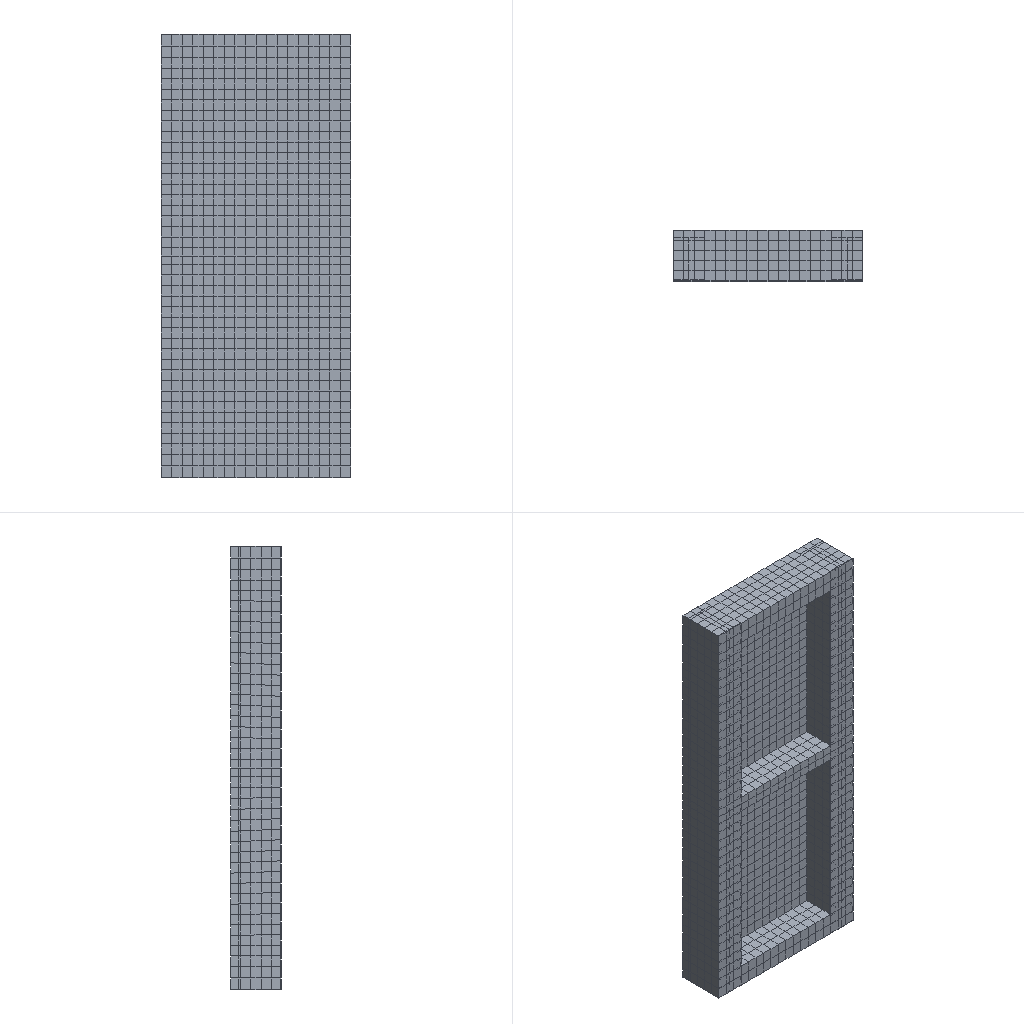Simulation study | abaqus
Set-up summary:
category,name,step,type,value,unit,region
solver,abaqus
solver,version,,,Abaqus/Explicit 2020
units,not stated in the deck,,not stated
analysis,deck,,transient,transient
load_step,Step-1,Step-1,transient
load_step,requested,,,1
mesh,nodes,,,5312
mesh,elements,,,3890
element_type,S4R,,shell,1008
element_type,T3D2,,truss,398
element_type,C3D8R,,solid,2484
load,load commands in deck,,count,1
bc,support commands in deck,,count,7
material,CON,,in results
material,STEEL,,in results
check,setup vs results,,match,"per instance, exact: element labels, types and connectivity; labels of the nodes the elements use; coordinates of those nodes at SINGLE_PRECISION in 19 of 19 instance(s)"
Abaqus input file, long lists of numbers shortened:
*Heading
** Job name: Job-3 Model name: Model-2-wangfu
** Generated by: Abaqus/CAE 2020
*Preprint, echo=NO, model=NO, history=NO, contact=NO
**
** PARTS
**
*Part, name=con
*Node
      1,         150.,           0.,        1090.
      2,         150.,           0.,        1350.
** (3778 more lines like these left out)
*Element, type=C3D8R
  1,    1,   73,  793,  106,  162,  849, 2683,  827
  2,   73,   74,  794,  793,  849,  850, 2684, 2683
** (2482 more lines like these left out)
*Nset, nset=Set-1, generate
    1,  3780,     1
*Elset, elset=Set-1, generate
    1,  2484,     1
** Section: con
*Solid Section, elset=Set-1, material=con
,
*End Part
**
*Part, name=gong
*Node
      1,           0.,           0.,           0.
      2,           0.,           0.,        2100.
** (557 more lines like these left out)
*Element, type=S4R
 1,   1,  13, 273,  96
 2,  13,  14, 274, 273
** (502 more lines like these left out)
*Nset, nset=Set-4
   1,   2,   7,   8,  13,  14,  15,  16,  17,  18,  19,  20,  21,  22,  23,  24
  25,  26,  27,  28,  29,  30,  31,  32,  33,  34,  35,  36,  37,  38,  39,  40
** (12 more lines like these left out)
*Elset, elset=Set-4, generate
 169,  336,    1
*Nset, nset=Set-5
   1,   2,   3,   4,   5,   6,   7,   8,   9,  10,  11,  12,  13,  14,  15,  16
  17,  18,  19,  20,  21,  22,  23,  24,  25,  26,  27,  28,  29,  30,  31,  32
** (25 more lines like these left out)
*Elset, elset=Set-5
   1,   2,   3,   4,   5,   6,   7,   8,   9,  10,  11,  12,  13,  14,  15,  16
  17,  18,  19,  20,  21,  22,  23,  24,  25,  26,  27,  28,  29,  30,  31,  32
** (19 more lines like these left out)
** Section: Section-heng
*Shell Section, elset=Set-5, material=steel
5., 5
** Section: Section-shu
*Shell Section, elset=Set-4, material=steel
4., 5
*End Part
**
*Part, name=xian
*Node
      1,           0.,           0.,           0.
      2,          50.,           0.,           0.
** (39 more lines like these left out)
*Element, type=T3D2
 1,  1,  2
 2,  2,  3
** (38 more lines like these left out)
*Nset, nset=Set-1, generate
  1,  41,   1
*Elset, elset=Set-1, generate
  1,  40,   1
** Section: xian
*Solid Section, elset=Set-1, material=steel
28.26,
*End Part
**
*Part, name=xian-ano
*Node
      1,           0.,         575.,           0.
      2,           0.,         525.,           0.
** (17 more lines like these left out)
*Element, type=T3D2
 1,  1,  2
 2,  2,  3
** (16 more lines like these left out)
*Nset, nset=Set-1, generate
  1,  19,   1
*Elset, elset=Set-1, generate
  1,  18,   1
** Section: xian
*Solid Section, elset=Set-1, material=steel
28.26,
*End Part
**
**
** ASSEMBLY
**
*Assembly, name=Assembly
**
*Instance, name=con-1, part=con
          0.,           0.,        2100.
*End Instance
**
*Instance, name=gong-2, part=gong
         75.,         -35.,        2100.
*End Instance
**
*Instance, name=gong-3, part=gong
        825.,         -35.,        2100.
*End Instance
**
*Instance, name=xian-1, part=xian
         51.,         -20.,        4145.
         51.,         -20.,        4145.,          51., -19.,        4145., 90.
*End Instance
**
*Instance, name=xian-1-lin-2-1, part=xian
        251.,         -20.,        4145.
        251.,         -20.,        4145.,         251., -19.,        4145., 90.
*End Instance
**
*Instance, name=xian-1-lin-3-1, part=xian
        451.,         -20.,        4145.
        451.,         -20.,        4145.,         451., -19.,        4145., 90.
*End Instance
**
*Instance, name=xian-1-lin-4-1, part=xian
        651.,         -20.,        4145.
        651.,         -20.,        4145.,         651., -19.,        4145., 90.
*End Instance
**
*Instance, name=xian-1-lin-5-1, part=xian
        851.,         -20.,        4145.
        851.,         -20.,        4145.,         851., -19.,        4145., 90.
*End Instance
**
*Instance, name=xian-ano-1, part=xian-ano
        575.,         -23.,        2145.
        575.,         -23.,        2145.,         575.,         -23., 2146., 90.
*End Instance
**
*Instance, name=xian-ano-1-lin-2-1, part=xian-ano
        575.,         -23.,        2345.
        575.,         -23.,        2345.,         575.,         -23., 2346., 90.
*End Instance
**
*Instance, name=xian-ano-1-lin-3-1, part=xian-ano
        575.,         -23.,        2545.
        575.,         -23.,        2545.,         575.,         -23., 2546., 90.
*End Instance
**
*Instance, name=xian-ano-1-lin-4-1, part=xian-ano
        575.,         -23.,        2745.
        575.,         -23.,        2745.,         575.,         -23., 2746., 90.
*End Instance
**
*Instance, name=xian-ano-1-lin-5-1, part=xian-ano
        575.,         -23.,        2945.
        575.,         -23.,        2945.,         575.,         -23., 2946., 90.
*End Instance
**
*Instance, name=xian-ano-1-lin-6-1, part=xian-ano
        575.,         -23.,        3145.
        575.,         -23.,        3145.,         575.,         -23., 3146., 90.
*End Instance
**
*Instance, name=xian-ano-1-lin-7-1, part=xian-ano
        575.,         -23.,        3345.
        575.,         -23.,        3345.,         575.,         -23., 3346., 90.
*End Instance
**
*Instance, name=xian-ano-1-lin-8-1, part=xian-ano
        575.,         -23.,        3545.
        575.,         -23.,        3545.,         575.,         -23., 3546., 90.
*End Instance
**
*Instance, name=xian-ano-1-lin-9-1, part=xian-ano
        575.,         -23.,        3745.
        575.,         -23.,        3745.,         575.,         -23., 3746., 90.
*End Instance
**
*Instance, name=xian-ano-1-lin-10-1, part=xian-ano
        575.,         -23.,        3945.
        575.,         -23.,        3945.,         575.,         -23., 3946., 90.
*End Instance
**
*Instance, name=xian-ano-1-lin-11-1, part=xian-ano
        575.,         -23.,        4145.
        575.,         -23.,        4145.,         575.,         -23., 4146., 90.
*End Instance
**
*Node
      1,         450.,           0.,        3150.
*Nset, nset=Set-2, instance=con-1
   29,   30,   32,   33,   35,   36,   44,   48,   50,   51,   54,   56,   59,   60,   61,   64
  375,  383,  391,  392,  393,  394,  395,  396,  397,  398,  399,  400,  401,  413,  414,  415
** (6 more lines like these left out)
*Elset, elset=Set-2, instance=con-1
  985,  986,  995,  996, 1005, 1006, 1015, 1016, 1025, 1026, 1035, 1036, 1045, 1046, 1055, 1056
 1065, 1066, 1075, 1076, 1085, 1086, 1095, 1096, 1675, 1676, 1685, 1686, 1695, 1696, 1705, 1706
** (3 more lines like these left out)
*Nset, nset=Set-3
 1,
*Nset, nset=m_Set-1
 1,
*Nset, nset=m_Set-4, instance=gong-2, generate
   1,  559,    1
*Nset, nset=m_Set-4, instance=gong-3, generate
   1,  559,    1
*Nset, nset=m_Set-4, instance=xian-1-lin-2-1, generate
  1,  41,   1
*Nset, nset=m_Set-4, instance=xian-ano-1, generate
  1,  19,   1
*Nset, nset=m_Set-4, instance=xian-ano-1-lin-5-1, generate
  1,  19,   1
*Nset, nset=m_Set-4, instance=xian-ano-1-lin-9-1, generate
  1,  19,   1
*Nset, nset=m_Set-4, instance=xian-1-lin-4-1, generate
  1,  41,   1
*Nset, nset=m_Set-4, instance=xian-ano-1-lin-7-1, generate
  1,  19,   1
*Nset, nset=m_Set-4, instance=xian-ano-1-lin-3-1, generate
  1,  19,   1
*Nset, nset=m_Set-4, instance=xian-ano-1-lin-11-1, generate
  1,  19,   1
*Nset, nset=m_Set-4, instance=xian-1, generate
  1,  41,   1
*Nset, nset=m_Set-4, instance=xian-1-lin-3-1, generate
  1,  41,   1
*Nset, nset=m_Set-4, instance=xian-ano-1-lin-6-1, generate
  1,  19,   1
*Nset, nset=m_Set-4, instance=xian-ano-1-lin-2-1, generate
  1,  19,   1
*Nset, nset=m_Set-4, instance=xian-ano-1-lin-10-1, generate
  1,  19,   1
*Nset, nset=m_Set-4, instance=xian-1-lin-5-1, generate
  1,  41,   1
*Nset, nset=m_Set-4, instance=xian-ano-1-lin-8-1, generate
  1,  19,   1
*Nset, nset=m_Set-4, instance=xian-ano-1-lin-4-1, generate
  1,  19,   1
*Elset, elset=m_Set-4, instance=gong-2, generate
   1,  504,    1
*Elset, elset=m_Set-4, instance=gong-3, generate
   1,  504,    1
*Elset, elset=m_Set-4, instance=xian-1-lin-2-1, generate
  1,  40,   1
*Elset, elset=m_Set-4, instance=xian-ano-1, generate
  1,  18,   1
*Elset, elset=m_Set-4, instance=xian-ano-1-lin-5-1, generate
  1,  18,   1
*Elset, elset=m_Set-4, instance=xian-ano-1-lin-9-1, generate
  1,  18,   1
*Elset, elset=m_Set-4, instance=xian-1-lin-4-1, generate
  1,  40,   1
*Elset, elset=m_Set-4, instance=xian-ano-1-lin-7-1, generate
  1,  18,   1
*Elset, elset=m_Set-4, instance=xian-ano-1-lin-3-1, generate
  1,  18,   1
*Elset, elset=m_Set-4, instance=xian-ano-1-lin-11-1, generate
  1,  18,   1
*Elset, elset=m_Set-4, instance=xian-1, generate
  1,  40,   1
*Elset, elset=m_Set-4, instance=xian-1-lin-3-1, generate
  1,  40,   1
*Elset, elset=m_Set-4, instance=xian-ano-1-lin-6-1, generate
  1,  18,   1
*Elset, elset=m_Set-4, instance=xian-ano-1-lin-2-1, generate
  1,  18,   1
*Elset, elset=m_Set-4, instance=xian-ano-1-lin-10-1, generate
  1,  18,   1
*Elset, elset=m_Set-4, instance=xian-1-lin-5-1, generate
  1,  40,   1
*Elset, elset=m_Set-4, instance=xian-ano-1-lin-8-1, generate
  1,  18,   1
*Elset, elset=m_Set-4, instance=xian-ano-1-lin-4-1, generate
  1,  18,   1
*Nset, nset=s_Set-4, instance=con-1, generate
    1,  3780,     1
*Elset, elset=s_Set-4, instance=con-1, generate
    1,  2484,     1
*Elset, elset=_s_Surf-1_S4, internal, instance=con-1
 1464, 1469, 1554, 1559, 1644, 1649
*Elset, elset=_s_Surf-1_S2, internal, instance=con-1
 1326, 1327, 1344, 1345, 1362, 1363, 2230, 2231, 2232, 2233, 2234, 2235
*Elset, elset=_s_Surf-1_S6, internal, instance=con-1
 1850, 1855, 1940, 1945, 2030, 2035
*Elset, elset=_s_Surf-1_S3, internal, instance=con-1
   6,   7,  42,  43,  78,  79, 114, 115, 150, 151, 186, 187, 222, 223, 258, 259
 294, 295, 330, 331, 366, 367, 402, 403
*Elset, elset=_s_Surf-1_S5, internal, instance=con-1
 576, 577, 612, 613, 648, 649, 684, 685, 720, 721, 756, 757, 792, 793, 828, 829
 864, 865, 900, 901, 936, 937, 972, 973
*Surface, type=ELEMENT, name=s_Surf-1
_s_Surf-1_S4, S4
_s_Surf-1_S2, S2
_s_Surf-1_S6, S6
_s_Surf-1_S3, S3
_s_Surf-1_S5, S5
** Constraint: Constraint-1
*Coupling, constraint name=Constraint-1, ref node=m_Set-1, surface=s_Surf-1
*Kinematic
** Constraint: Constraint-2
*Embedded Element, host elset=s_Set-4
m_Set-4
*End Assembly
*Amplitude, name=Amp-1
             0.,              0.,              1.,              1.
*Amplitude, name=Amp-2, definition=PERIODIC
1,           0.628,              0.,              0.
            35.,              0.
*Amplitude, name=Amp-3
             0.,              0.,             0.1,              5.,             0.2,              0.,             0.3,             -5.
            0.4,              0.,             0.5,             10.,             0.6,              0.,             0.7,            -10.
            0.8,              0.,             0.9,             15.,              1.,              0.,             1.1,            -15.
            1.2,              0.,             1.3,             20.,             1.4,              0.,             1.5,            -20.
            1.6,              0.
**
** MATERIALS
**
*Material, name=con
*Density
 2.5e-09,
*Elastic
32500., 0.2
*Concrete Damaged Plasticity
30.,   0.1,  1.16, 0.667,  0.01
*Concrete Compression Hardening
 31.839,          0.
  35.238, 0.0001688
  37.656, 0.0002734
 39.058, 0.0004092
    39.5, 0.0005746
 38.815, 0.0007747
 37.101,  0.001006
  34.823,  0.001256
 32.332,  0.001511
 29.849,  0.001767
 27.497,  0.002018
 25.334,   0.002263
 23.376,  0.002503
 21.619,  0.002736
 20.051,  0.002963
 18.651,  0.003185
 17.402,  0.003403
 16.285,  0.003616
 15.284,  0.003826
 14.385,   0.004032
 13.573,  0.004236
 12.839,  0.004438
 12.173,  0.004637
 11.567,   0.004835
  11.013,  0.005031
*Concrete Tension Stiffening
  2.09,       0.
   2.4, 8.74e-06
  2.67, 1.23e-05
  2.86, 1.81e-05
  2.94, 2.75e-05
   2.8, 4.37e-05
  2.55, 6.31e-05
   2.3, 8.27e-05
  2.07, 0.000102
  1.86,  0.00012
  1.69, 0.000137
  1.55, 0.000153
  1.42, 0.000169
  1.31, 0.000184
  1.22, 0.000198
  1.14, 0.000213
  1.07, 0.000227
  1.01,  0.00024
 0.956, 0.000254
 0.908, 0.000267
 0.864,  0.00028
 0.825, 0.000293
 0.789, 0.000306
 0.757, 0.000319
 0.727, 0.000332
*Concrete Compression Damage
        0.,          0.
 0.06977, 0.0001688
  0.1005, 0.0002734
  0.1363, 0.0004092
  0.176, 0.0005746
  0.2212, 0.0007747
  0.271,  0.001006
  0.3214,  0.001256
  0.3699,  0.001511
  0.4151,  0.001767
  0.4565,  0.002018
  0.4939,   0.002263
  0.5275,  0.002503
   0.5577,  0.002736
  0.5849,  0.002963
   0.6093,  0.003185
  0.6313,  0.003403
  0.6511,  0.003616
  0.6691,  0.003826
  0.6855,   0.004032
  0.7004,  0.004236
  0.7141,  0.004438
  0.7266,  0.004637
  0.7382,   0.004835
  0.7488,  0.005031
  0.7586,  0.005226
  0.7678,  0.005419
  0.7763,  0.005611
  0.7842,  0.005802
  0.7915,  0.005993
  0.7984,  0.006182
  0.8049,  0.006371
  0.811,  0.006559
  0.8167,  0.006747
  0.8221,  0.006933
  0.8627,  0.008781
  0.8884,   0.01061
  0.906,   0.01242
  0.9188,   0.01423
  0.9286,   0.01603
** (21 more lines like these left out)
*Concrete Tension Damage, compression recovery=0.45
     0.,       0.
 0.0544, 8.74e-06
 0.0674, 1.23e-05
 0.0893, 1.81e-05
  0.124, 2.75e-05
  0.186, 4.37e-05
  0.255, 6.31e-05
  0.321, 8.27e-05
   0.38, 0.000102
  0.431,  0.00012
  0.475, 0.000137
  0.513, 0.000153
  0.546, 0.000169
  0.575, 0.000184
  0.601, 0.000198
  0.623, 0.000213
  0.643, 0.000227
  0.661,  0.00024
  0.678, 0.000254
  0.692, 0.000267
  0.706,  0.00028
  0.718, 0.000293
  0.729, 0.000306
  0.739, 0.000319
  0.749, 0.000332
  0.757, 0.000344
  0.765, 0.000357
  0.773, 0.000369
   0.78, 0.000382
  0.787, 0.000394
  0.793, 0.000407
  0.799, 0.000419
  0.804, 0.000431
  0.809, 0.000443
  0.814, 0.000456
  0.851, 0.000577
  0.875, 0.000697
  0.892, 0.000816
  0.905, 0.000935
  0.915,  0.00105
** (31 more lines like these left out)
*Material, name=steel
*Density
 7.8e-09,
*Elastic
210000., 0.3
*Plastic
320.,0.
** ----------------------------------------------------------------
**
** STEP: Step-1
**
*Step, name=Step-1, nlgeom=YES
*Dynamic, Explicit
, 1.6
*Bulk Viscosity
0.06, 1.2
**
** BOUNDARY CONDITIONS
**
** Name: BC-1 Type: 位移/转角
*Boundary
Set-2, 2, 2
** Name: [REDACTED] : Displacement/rotation angle
*Boundary, amplitude=Amp-3
Set-3, 1, 1
Set-3, 2, 2, -1.
Set-3, 3, 3
Set-3, 4, 4
Set-3, 5, 5
Set-3, 6, 6
**
** OUTPUT REQUESTS
**
*Restart, write, number interval=1, time marks=NO
**
** FIELD OUTPUT: F-Output-1
**
*Output, field, number interval=50
*Node Output
CF, RF, RM, RT, U, V
*Element Output, directions=YES
DAMAGEC, DAMAGET, E, LE, MISES, MISESMAX, MISESONLY, PE, PEEQ, PEEQMAX, PEEQT, PEMAG, PRESSONLY, S, SDEG, SSAVG
TSHR, YIELDPOT
*Element Output, rebar, directions=YES
DAMAGEC, DAMAGET, E, LE, MISES, MISESMAX, MISESONLY, PE, PEEQ, PEEQMAX, PEEQT, PEMAG, PRESSONLY, RBANG, RBFOR, RBROT
S, SDEG, SSAVG, TSHR, YIELDPOT
*Contact Output
CDISP, CSTRESS
**
** HISTORY OUTPUT: H-Output-1
**
*Output, history, time interval=3.2e-05
*Node Output, nset=Set-3
RF2, U2
*End Step
Results summary:
result,step,Step-1,completed,increments=270117 time=1.6/1.6
result,analysis,,,transient
result,last_loadstep,,,1
result,primary field,,,"U, UR"
result,reaction total,,FX,-1587.18,model units
result,reaction total,,FY,3331.545,model units
result,reaction total,,FZ,-3253.203,model units